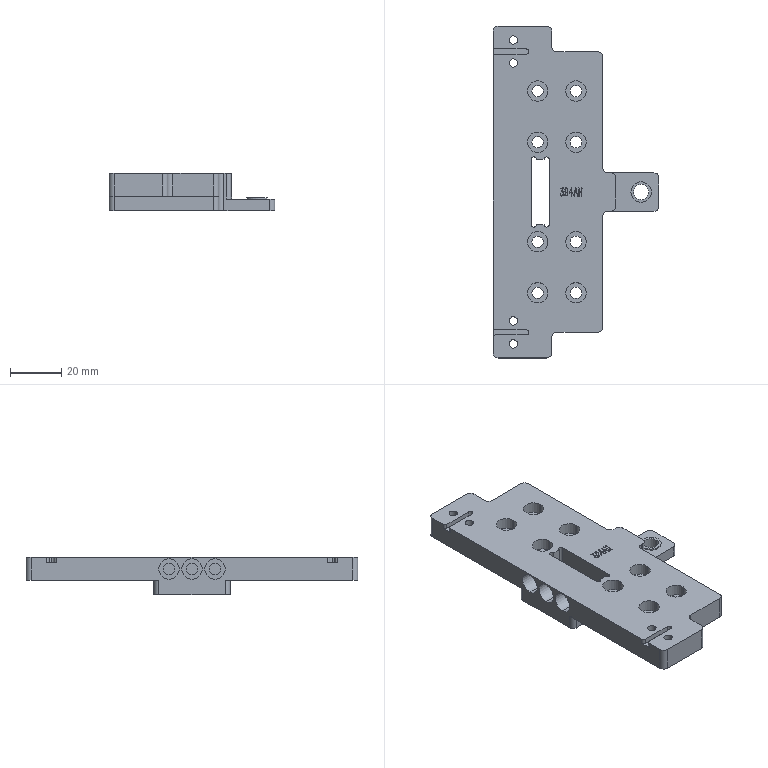NC program | NX | posted with a generic post | part box 65 x 130 x 14.5 mm
Lines 2037 to 2961 of 11541:
(ZLEVEL_PROFILE_COPY_COPY_COPY_1 , TOOL : D3)
N4036 T16 M6
N4038 G54
N4040 G17 G0 G90 X9.873 Y12.6 B0. C0. S9500 M3
N4042 G43 Z30. H16
N4044 Z-0.149
N4046 G94 G1 X10.133 Y12.15 F1000.
N4048 G3 X10.393 Y12. R0.3
N4050 G1 X11.336 F1200.
N4052 G2 X11.25 Y12.5 R1.5
N4054 G1 Y12.876
N4056 G3 X11.1 Y13.136 R0.3
N4058 G1 X10.65 Y13.396
N4060 G0 X9.873 Y12.6 Z-0.299
N4062 G1 X10.133 Y12.15 F1000.
N4064 G3 X10.393 Y12. R0.3
N4066 G1 X11.336 F1200.
N4068 G2 X11.25 Y12.5 R1.5
N4070 G1 Y12.876
N4072 G3 X11.1 Y13.136 R0.3
N4074 G1 X10.65 Y13.396
N4076 G0 X9.873 Y12.6 Z-0.448
N4078 G1 X10.133 Y12.15 F1000.
N4080 G3 X10.393 Y12. R0.3
N4082 G1 X11.336 F1200.
N4084 G2 X11.25 Y12.5 R1.5
N4086 G1 Y12.876
N4088 G3 X11.1 Y13.136 R0.3
N4090 G1 X10.65 Y13.396
N4092 G0 X9.873 Y12.6 Z-0.598
N4094 G1 X10.133 Y12.15 F1000.
N4096 G3 X10.393 Y12. R0.3
N4098 G1 X11.336 F1200.
N4100 G2 X11.25 Y12.5 R1.5
N4102 G1 Y12.876
N4104 G3 X11.1 Y13.136 R0.3
N4106 G1 X10.65 Y13.396
N4108 G0 X9.873 Y12.6 Z-0.747
N4110 G1 X10.133 Y12.15 F1000.
N4112 G3 X10.393 Y12. R0.3
N4114 G1 X11.336 F1200.
N4116 G2 X11.25 Y12.5 R1.5
N4118 G1 Y12.876
N4120 G3 X11.1 Y13.136 R0.3
N4122 G1 X10.65 Y13.396
N4124 G0 X9.873 Y12.6 Z-0.897
N4126 G1 X10.133 Y12.15 F1000.
N4128 G3 X10.393 Y12. R0.3
N4130 G1 X11.336 F1200.
N4132 G2 X11.25 Y12.5 R1.5
N4134 G1 Y12.876
N4136 G3 X11.1 Y13.136 R0.3
N4138 G1 X10.65 Y13.396
N4140 G0 X9.873 Y12.6 Z-1.046
N4142 G1 X10.133 Y12.15 F1000.
N4144 G3 X10.393 Y12. R0.3
N4146 G1 X11.336 F1200.
N4148 G2 X11.25 Y12.5 R1.5
N4150 G1 Y12.876
N4152 G3 X11.1 Y13.136 R0.3
N4154 G1 X10.65 Y13.396
N4156 G0 X9.873 Y12.6 Z-1.196
N4158 G1 X10.133 Y12.15 F1000.
N4160 G3 X10.393 Y12. R0.3
N4162 G1 X11.336 F1200.
N4164 G2 X11.25 Y12.5 R1.5
N4166 G1 Y12.876
N4168 G3 X11.1 Y13.136 R0.3
N4170 G1 X10.65 Y13.396
N4172 G0 X9.873 Y12.6 Z-1.345
N4174 G1 X10.133 Y12.15 F1000.
N4176 G3 X10.393 Y12. R0.3
N4178 G1 X11.336 F1200.
N4180 G2 X11.25 Y12.5 R1.5
N4182 G1 Y12.876
N4184 G3 X11.1 Y13.136 R0.3
N4186 G1 X10.65 Y13.396
N4188 G0 X9.873 Y12.6 Z-1.495
N4190 G1 X10.133 Y12.15 F1000.
N4192 G3 X10.393 Y12. R0.3
N4194 G1 X11.336 F1200.
N4196 G2 X11.25 Y12.5 R1.5
N4198 G1 Y12.876
N4200 G3 X11.1 Y13.136 R0.3
N4202 G1 X10.65 Y13.396
N4204 G0 X9.873 Y12.6 Z-1.644
N4206 G1 X10.133 Y12.15 F1000.
N4208 G3 X10.393 Y12. R0.3
N4210 G1 X11.336 F1200.
N4212 G2 X11.25 Y12.5 R1.5
N4214 G1 Y12.876
N4216 G3 X11.1 Y13.136 R0.3
N4218 G1 X10.65 Y13.396
N4220 G0 X9.873 Y12.6 Z-1.794
N4222 G1 X10.133 Y12.15 F1000.
N4224 G3 X10.393 Y12. R0.3
N4226 G1 X11.336 F1200.
N4228 G2 X11.25 Y12.5 R1.5
N4230 G1 Y12.876
N4232 G3 X11.1 Y13.136 R0.3
N4234 G1 X10.65 Y13.396
N4236 G0 X9.873 Y12.6 Z-1.943
N4238 G1 X10.133 Y12.15 F1000.
N4240 G3 X10.393 Y12. R0.3
N4242 G1 X11.336 F1200.
N4244 G2 X11.25 Y12.5 R1.5
N4246 G1 Y12.876
N4248 G3 X11.1 Y13.136 R0.3
N4250 G1 X10.65 Y13.396
N4252 G0 X9.873 Y12.6 Z-2.093
N4254 G1 X10.133 Y12.15 F1000.
N4256 G3 X10.393 Y12. R0.3
N4258 G1 X11.336 F1200.
N4260 G2 X11.25 Y12.5 R1.5
N4262 G1 Y12.876
N4264 G3 X11.1 Y13.136 R0.3
N4266 G1 X10.65 Y13.396
N4268 G0 X9.873 Y12.6 Z-2.242
N4270 G1 X10.133 Y12.15 F1000.
N4272 G3 X10.393 Y12. R0.3
N4274 G1 X11.336 F1200.
N4276 G2 X11.25 Y12.5 R1.5
N4278 G1 Y12.876
N4280 G3 X11.1 Y13.136 R0.3
N4282 G1 X10.65 Y13.396
N4284 G0 X9.873 Y12.6 Z-2.392
N4286 G1 X10.133 Y12.15 F1000.
N4288 G3 X10.393 Y12. R0.3
N4290 G1 X11.336 F1200.
N4292 G2 X11.25 Y12.5 R1.5
N4294 G1 Y12.876
N4296 G3 X11.1 Y13.136 R0.3
N4298 G1 X10.65 Y13.396
N4300 G0 X9.873 Y12.6 Z-2.541
N4302 G1 X10.133 Y12.15 F1000.
N4304 G3 X10.393 Y12. R0.3
N4306 G1 X11.336 F1200.
N4308 G2 X11.25 Y12.5 R1.5
N4310 G1 Y12.876
N4312 G3 X11.1 Y13.136 R0.3
N4314 G1 X10.65 Y13.396
N4316 G0 X9.873 Y12.6 Z-2.691
N4318 G1 X10.133 Y12.15 F1000.
N4320 G3 X10.393 Y12. R0.3
N4322 G1 X11.336 F1200.
N4324 G2 X11.25 Y12.5 R1.5
N4326 G1 Y12.876
N4328 G3 X11.1 Y13.136 R0.3
N4330 G1 X10.65 Y13.396
N4332 G0 X9.873 Y12.6 Z-2.84
N4334 G1 X10.133 Y12.15 F1000.
N4336 G3 X10.393 Y12. R0.3
N4338 G1 X11.336 F1200.
N4340 G2 X11.25 Y12.5 R1.5
N4342 G1 Y12.876
N4344 G3 X11.1 Y13.136 R0.3
N4346 G1 X10.65 Y13.396
N4348 G0 X9.873 Y12.6 Z-2.99
N4350 G1 X10.133 Y12.15 F1000.
N4352 G3 X10.393 Y12. R0.3
N4354 G1 X11.336 F1200.
N4356 G2 X11.25 Y12.5 R1.5
N4358 G1 Y12.876
N4360 G3 X11.1 Y13.136 R0.3
N4362 G1 X10.65 Y13.396
N4364 G0 X9.873 Y12.6 Z-3.139
N4366 G1 X10.133 Y12.15 F1000.
N4368 G3 X10.393 Y12. R0.3
N4370 G1 X11.336 F1200.
N4372 G2 X11.25 Y12.5 R1.5
N4374 G1 Y12.876
N4376 G3 X11.1 Y13.136 R0.3
N4378 G1 X10.65 Y13.396
N4380 G0 X9.873 Y12.6 Z-3.289
N4382 G1 X10.133 Y12.15 F1000.
N4384 G3 X10.393 Y12. R0.3
N4386 G1 X11.336 F1200.
N4388 G2 X11.25 Y12.5 R1.5
N4390 G1 Y12.876
N4392 G3 X11.1 Y13.136 R0.3
N4394 G1 X10.65 Y13.396
N4396 G0 X9.873 Y12.6 Z-3.438
N4398 G1 X10.133 Y12.15 F1000.
N4400 G3 X10.393 Y12. R0.3
N4402 G1 X11.336 F1200.
N4404 G2 X11.25 Y12.5 R1.5
N4406 G1 Y12.876
N4408 G3 X11.1 Y13.136 R0.3
N4410 G1 X10.65 Y13.396
N4412 G0 X9.873 Y12.6 Z-3.588
N4414 G1 X10.133 Y12.15 F1000.
N4416 G3 X10.393 Y12. R0.3
N4418 G1 X11.336 F1200.
N4420 G2 X11.25 Y12.5 R1.5
N4422 G1 Y12.876
N4424 G3 X11.1 Y13.136 R0.3
N4426 G1 X10.65 Y13.396
N4428 G0 X9.873 Y12.6 Z-3.737
N4430 G1 X10.133 Y12.15 F1000.
N4432 G3 X10.393 Y12. R0.3
N4434 G1 X11.336 F1200.
N4436 G2 X11.25 Y12.5 R1.5
N4438 G1 Y12.876
N4440 G3 X11.1 Y13.136 R0.3
N4442 G1 X10.65 Y13.396
N4444 G0 X9.873 Y12.6 Z-3.887
N4446 G1 X10.133 Y12.15 F1000.
N4448 G3 X10.393 Y12. R0.3
N4450 G1 X11.336 F1200.
N4452 G2 X11.25 Y12.5 R1.5
N4454 G1 Y12.876
N4456 G3 X11.1 Y13.136 R0.3
N4458 G1 X10.65 Y13.396
N4460 G0 X9.873 Y12.6 Z-4.036
N4462 G1 X10.133 Y12.15 F1000.
N4464 G3 X10.393 Y12. R0.3
N4466 G1 X11.336 F1200.
N4468 G2 X11.25 Y12.5 R1.5
N4470 G1 Y12.876
N4472 G3 X11.1 Y13.136 R0.3
N4474 G1 X10.65 Y13.396
N4476 G0 X9.873 Y12.6 Z-4.186
N4478 G1 X10.133 Y12.15 F1000.
N4480 G3 X10.393 Y12. R0.3
N4482 G1 X11.336 F1200.
N4484 G2 X11.25 Y12.5 R1.5
N4486 G1 Y12.876
N4488 G3 X11.1 Y13.136 R0.3
N4490 G1 X10.65 Y13.396
N4492 G0 X9.873 Y12.6 Z-4.335
N4494 G1 X10.133 Y12.15 F1000.
N4496 G3 X10.393 Y12. R0.3
N4498 G1 X11.336 F1200.
N4500 G2 X11.25 Y12.5 R1.5
N4502 G1 Y12.876
N4504 G3 X11.1 Y13.136 R0.3
N4506 G1 X10.65 Y13.396
N4508 G0 X9.873 Y12.6 Z-4.485
N4510 G1 X10.133 Y12.15 F1000.
N4512 G3 X10.393 Y12. R0.3
N4514 G1 X11.336 F1200.
N4516 G2 X11.25 Y12.5 R1.5
N4518 G1 Y12.876
N4520 G3 X11.1 Y13.136 R0.3
N4522 G1 X10.65 Y13.396
N4524 G0 X9.873 Y12.6 Z-4.634
N4526 G1 X10.133 Y12.15 F1000.
N4528 G3 X10.393 Y12. R0.3
N4530 G1 X11.336 F1200.
N4532 G2 X11.25 Y12.5 R1.5
N4534 G1 Y12.876
N4536 G3 X11.1 Y13.136 R0.3
N4538 G1 X10.65 Y13.396
N4540 G0 X9.873 Y12.6 Z-4.784
N4542 G1 X10.133 Y12.15 F1000.
N4544 G3 X10.393 Y12. R0.3
N4546 G1 X11.336 F1200.
N4548 G2 X11.25 Y12.5 R1.5
N4550 G1 Y12.876
N4552 G3 X11.1 Y13.136 R0.3
N4554 G1 X10.65 Y13.396
N4556 G0 X9.873 Y12.6 Z-4.933
N4558 G1 X10.133 Y12.15 F1000.
N4560 G3 X10.393 Y12. R0.3
N4562 G1 X11.336 F1200.
N4564 G2 X11.25 Y12.5 R1.5
N4566 G1 Y12.876
N4568 G3 X11.1 Y13.136 R0.3
N4570 G1 X10.65 Y13.396
N4572 G0 X9.873 Y12.6 Z-5.082
N4574 G1 X10.133 Y12.15 F1000.
N4576 G3 X10.393 Y12. R0.3
N4578 G1 X11.336 F1200.
N4580 G2 X11.25 Y12.5 R1.5
N4582 G1 Y12.876
N4584 G3 X11.1 Y13.136 R0.3
N4586 G1 X10.65 Y13.396
N4588 G0 X9.873 Y12.6 Z-5.232
N4590 G1 X10.133 Y12.15 F1000.
N4592 G3 X10.393 Y12. R0.3
N4594 G1 X11.336 F1200.
N4596 G2 X11.25 Y12.5 R1.5
N4598 G1 Y12.876
N4600 G3 X11.1 Y13.136 R0.3
N4602 G1 X10.65 Y13.396
N4604 G0 X9.873 Y12.6 Z-5.381
N4606 G1 X10.133 Y12.15 F1000.
N4608 G3 X10.393 Y12. R0.3
N4610 G1 X11.336 F1200.
N4612 G2 X11.25 Y12.5 R1.5
N4614 G1 Y12.876
N4616 G3 X11.1 Y13.136 R0.3
N4618 G1 X10.65 Y13.396
N4620 G0 X9.873 Y12.6 Z-5.531
N4622 G1 X10.133 Y12.15 F1000.
N4624 G3 X10.393 Y12. R0.3
N4626 G1 X11.336 F1200.
N4628 G2 X11.25 Y12.5 R1.5
N4630 G1 Y12.876
N4632 G3 X11.1 Y13.136 R0.3
N4634 G1 X10.65 Y13.396
N4636 G0 X9.873 Y12.6 Z-5.68
N4638 G1 X10.133 Y12.15 F1000.
N4640 G3 X10.393 Y12. R0.3
N4642 G1 X11.336 F1200.
N4644 G2 X11.25 Y12.5 R1.5
N4646 G1 Y12.876
N4648 G3 X11.1 Y13.136 R0.3
N4650 G1 X10.65 Y13.396
N4652 G0 X9.873 Y12.6 Z-5.83
N4654 G1 X10.133 Y12.15 F1000.
N4656 G3 X10.393 Y12. R0.3
N4658 G1 X11.336 F1200.
N4660 G2 X11.25 Y12.5 R1.5
N4662 G1 Y12.876
N4664 G3 X11.1 Y13.136 R0.3
N4666 G1 X10.65 Y13.396
N4668 G0 X9.873 Y12.6 Z-5.979
N4670 G1 X10.133 Y12.15 F1000.
N4672 G3 X10.393 Y12. R0.3
N4674 G1 X11.336 F1200.
N4676 G2 X11.25 Y12.5 R1.5
N4678 G1 Y12.876
N4680 G3 X11.1 Y13.136 R0.3
N4682 G1 X10.65 Y13.396
N4684 G0 X9.873 Y12.6 Z-6.129
N4686 G1 X10.133 Y12.15 F1000.
N4688 G3 X10.393 Y12. R0.3
N4690 G1 X11.336 F1200.
N4692 G2 X11.25 Y12.5 R1.5
N4694 G1 Y12.876
N4696 G3 X11.1 Y13.136 R0.3
N4698 G1 X10.65 Y13.396
N4700 G0 X9.873 Y12.6 Z-6.278
N4702 G1 X10.133 Y12.15 F1000.
N4704 G3 X10.393 Y12. R0.3
N4706 G1 X11.336 F1200.
N4708 G2 X11.25 Y12.5 R1.5
N4710 G1 Y12.876
N4712 G3 X11.1 Y13.136 R0.3
N4714 G1 X10.65 Y13.396
N4716 G0 X9.873 Y12.6 Z-6.428
N4718 G1 X10.133 Y12.15 F1000.
N4720 G3 X10.393 Y12. R0.3
N4722 G1 X11.336 F1200.
N4724 G2 X11.25 Y12.5 R1.5
N4726 G1 Y12.876
N4728 G3 X11.1 Y13.136 R0.3
N4730 G1 X10.65 Y13.396
N4732 G0 X9.873 Y12.6 Z-6.577
N4734 G1 X10.133 Y12.15 F1000.
N4736 G3 X10.393 Y12. R0.3
N4738 G1 X11.336 F1200.
N4740 G2 X11.25 Y12.5 R1.5
N4742 G1 Y12.876
N4744 G3 X11.1 Y13.136 R0.3
N4746 G1 X10.65 Y13.396
N4748 G0 X9.873 Y12.6 Z-6.727
N4750 G1 X10.133 Y12.15 F1000.
N4752 G3 X10.393 Y12. R0.3
N4754 G1 X11.336 F1200.
N4756 G2 X11.25 Y12.5 R1.5
N4758 G1 Y12.876
N4760 G3 X11.1 Y13.136 R0.3
N4762 G1 X10.65 Y13.396
N4764 G0 X9.873 Y12.6 Z-6.876
N4766 G1 X10.133 Y12.15 F1000.
N4768 G3 X10.393 Y12. R0.3
N4770 G1 X11.336 F1200.
N4772 G2 X11.25 Y12.5 R1.5
N4774 G1 Y12.876
N4776 G3 X11.1 Y13.136 R0.3
N4778 G1 X10.65 Y13.396
N4780 G0 X9.873 Y12.6 Z-7.026
N4782 G1 X10.133 Y12.15 F1000.
N4784 G3 X10.393 Y12. R0.3
N4786 G1 X11.336 F1200.
N4788 G2 X11.25 Y12.5 R1.5
N4790 G1 Y12.876
N4792 G3 X11.1 Y13.136 R0.3
N4794 G1 X10.65 Y13.396
N4796 G0 X9.873 Y12.6 Z-7.175
N4798 G1 X10.133 Y12.15 F1000.
N4800 G3 X10.393 Y12. R0.3
N4802 G1 X11.336 F1200.
N4804 G2 X11.25 Y12.5 R1.5
N4806 G1 Y12.876
N4808 G3 X11.1 Y13.136 R0.3
N4810 G1 X10.65 Y13.396
N4812 G0 X9.873 Y12.6 Z-7.325
N4814 G1 X10.133 Y12.15 F1000.
N4816 G3 X10.393 Y12. R0.3
N4818 G1 X11.336 F1200.
N4820 G2 X11.25 Y12.5 R1.5
N4822 G1 Y12.876
N4824 G3 X11.1 Y13.136 R0.3
N4826 G1 X10.65 Y13.396
N4828 G0 X9.873 Y12.6 Z-7.474
N4830 G1 X10.133 Y12.15 F1000.
N4832 G3 X10.393 Y12. R0.3
N4834 G1 X11.336 F1200.
N4836 G2 X11.25 Y12.5 R1.5
N4838 G1 Y12.876
N4840 G3 X11.1 Y13.136 R0.3
N4842 G1 X10.65 Y13.396
N4844 G0 X9.873 Y12.6 Z-7.624
N4846 G1 X10.133 Y12.15 F1000.
N4848 G3 X10.393 Y12. R0.3
N4850 G1 X11.336 F1200.
N4852 G2 X11.25 Y12.5 R1.5
N4854 G1 Y12.876
N4856 G3 X11.1 Y13.136 R0.3
N4858 G1 X10.65 Y13.396
N4860 G0 X9.873 Y12.6 Z-7.773
N4862 G1 X10.133 Y12.15 F1000.
N4864 G3 X10.393 Y12. R0.3
N4866 G1 X11.336 F1200.
N4868 G2 X11.25 Y12.5 R1.5
N4870 G1 Y12.876
N4872 G3 X11.1 Y13.136 R0.3
N4874 G1 X10.65 Y13.396
N4876 G0 X9.873 Y12.6 Z-7.923
N4878 G1 X10.133 Y12.15 F1000.
N4880 G3 X10.393 Y12. R0.3
N4882 G1 X11.336 F1200.
N4884 G2 X11.25 Y12.5 R1.5
N4886 G1 Y12.876
N4888 G3 X11.1 Y13.136 R0.3
N4890 G1 X10.65 Y13.396
N4892 G0 X9.873 Y12.6 Z-8.072
N4894 G1 X10.133 Y12.15 F1000.
N4896 G3 X10.393 Y12. R0.3
N4898 G1 X11.336 F1200.
N4900 G2 X11.25 Y12.5 R1.5
N4902 G1 Y12.876
N4904 G3 X11.1 Y13.136 R0.3
N4906 G1 X10.65 Y13.396
N4908 G0 X9.873 Y12.6 Z-8.222
N4910 G1 X10.133 Y12.15 F1000.
N4912 G3 X10.393 Y12. R0.3
N4914 G1 X11.336 F1200.
N4916 G2 X11.25 Y12.5 R1.5
N4918 G1 Y12.876
N4920 G3 X11.1 Y13.136 R0.3
N4922 G1 X10.65 Y13.396
N4924 G0 X9.873 Y12.6 Z-8.371
N4926 G1 X10.133 Y12.15 F1000.
N4928 G3 X10.393 Y12. R0.3
N4930 G1 X11.336 F1200.
N4932 G2 X11.25 Y12.5 R1.5
N4934 G1 Y12.876
N4936 G3 X11.1 Y13.136 R0.3
N4938 G1 X10.65 Y13.396
N4940 G0 X9.873 Y12.6 Z-8.521
N4942 G1 X10.133 Y12.15 F1000.
N4944 G3 X10.393 Y12. R0.3
N4946 G1 X11.336 F1200.
N4948 G2 X11.25 Y12.5 R1.5
N4950 G1 Y12.876
N4952 G3 X11.1 Y13.136 R0.3
N4954 G1 X10.65 Y13.396
N4956 G0 X9.873 Y12.6 Z-8.67
N4958 G1 X10.133 Y12.15 F1000.
N4960 G3 X10.393 Y12. R0.3
N4962 G1 X11.336 F1200.
N4964 G2 X11.25 Y12.5 R1.5
N4966 G1 Y12.876
N4968 G3 X11.1 Y13.136 R0.3
N4970 G1 X10.65 Y13.396
N4972 G0 X9.873 Y12.6 Z-8.82
N4974 G1 X10.133 Y12.15 F1000.
N4976 G3 X10.393 Y12. R0.3
N4978 G1 X11.336 F1200.
N4980 G2 X11.25 Y12.5 R1.5
N4982 G1 Y12.876
N4984 G3 X11.1 Y13.136 R0.3
N4986 G1 X10.65 Y13.396
N4988 G0 X9.873 Y12.6 Z-8.969
N4990 G1 X10.133 Y12.15 F1000.
N4992 G3 X10.393 Y12. R0.3
N4994 G1 X11.336 F1200.
N4996 G2 X11.25 Y12.5 R1.5
N4998 G1 Y12.876
N5000 G3 X11.1 Y13.136 R0.3
N5002 G1 X10.65 Y13.396
N5004 G0 X9.873 Y12.6 Z-9.119
N5006 G1 X10.133 Y12.15 F1000.
N5008 G3 X10.393 Y12. R0.3
N5010 G1 X11.336 F1200.
N5012 G2 X11.25 Y12.5 R1.5
N5014 G1 Y12.876
N5016 G3 X11.1 Y13.136 R0.3
N5018 G1 X10.65 Y13.396
N5020 G0 X9.873 Y12.6 Z-9.268
N5022 G1 X10.133 Y12.15 F1000.
N5024 G3 X10.393 Y12. R0.3
N5026 G1 X11.336 F1200.
N5028 G2 X11.25 Y12.5 R1.5
N5030 G1 Y12.876
N5032 G3 X11.1 Y13.136 R0.3
N5034 G1 X10.65 Y13.396
N5036 G0 X9.873 Y12.6 Z-9.418
N5038 G1 X10.133 Y12.15 F1000.
N5040 G3 X10.393 Y12. R0.3
N5042 G1 X11.336 F1200.
N5044 G2 X11.25 Y12.5 R1.5
N5046 G1 Y12.876
N5048 G3 X11.1 Y13.136 R0.3
N5050 G1 X10.65 Y13.396
N5052 G0 X9.873 Y12.6 Z-9.567
N5054 G1 X10.133 Y12.15 F1000.
N5056 G3 X10.393 Y12. R0.3
N5058 G1 X11.336 F1200.
N5060 G2 X11.25 Y12.5 R1.5
N5062 G1 Y12.876
N5064 G3 X11.1 Y13.136 R0.3
N5066 G1 X10.65 Y13.396
N5068 G0 X9.873 Y12.6 Z-9.716
N5070 G1 X10.133 Y12.15 F1000.
N5072 G3 X10.393 Y12. R0.3
N5074 G1 X11.336 F1200.
N5076 G2 X11.25 Y12.5 R1.5
N5078 G1 Y12.876
N5080 G3 X11.1 Y13.136 R0.3
N5082 G1 X10.65 Y13.396
N5084 G0 X9.873 Y12.6 Z-9.866
N5086 G1 X10.133 Y12.15 F1000.
N5088 G3 X10.393 Y12. R0.3
N5090 G1 X11.336 F1200.
N5092 G2 X11.25 Y12.5 R1.5
N5094 G1 Y12.876
N5096 G3 X11.1 Y13.136 R0.3
N5098 G1 X10.65 Y13.396
N5100 G0 X9.873 Y12.6 Z-10.015
N5102 G1 X10.133 Y12.15 F1000.
N5104 G3 X10.393 Y12. R0.3
N5106 G1 X11.336 F1200.
N5108 G2 X11.25 Y12.5 R1.5
N5110 G1 Y12.876
N5112 G3 X11.1 Y13.136 R0.3
N5114 G1 X10.65 Y13.396
N5116 G0 X9.873 Y12.6 Z-10.165
N5118 G1 X10.133 Y12.15 F1000.
N5120 G3 X10.393 Y12. R0.3
N5122 G1 X11.336 F1200.
N5124 G2 X11.25 Y12.5 R1.5
N5126 G1 Y12.876
N5128 G3 X11.1 Y13.136 R0.3
N5130 G1 X10.65 Y13.396
N5132 G0 X9.873 Y12.6 Z-10.314
N5134 G1 X10.133 Y12.15 F1000.
N5136 G3 X10.393 Y12. R0.3
N5138 G1 X11.336 F1200.
N5140 G2 X11.25 Y12.5 R1.5
N5142 G1 Y12.876
N5144 G3 X11.1 Y13.136 R0.3
N5146 G1 X10.65 Y13.396
N5148 G0 X9.873 Y12.6 Z-10.464
N5150 G1 X10.133 Y12.15 F1000.
N5152 G3 X10.393 Y12. R0.3
N5154 G1 X11.336 F1200.
N5156 G2 X11.25 Y12.5 R1.5
N5158 G1 Y12.876
N5160 G3 X11.1 Y13.136 R0.3
N5162 G1 X10.65 Y13.396
N5164 G0 X9.873 Y12.6 Z-10.613
N5166 G1 X10.133 Y12.15 F1000.
N5168 G3 X10.393 Y12. R0.3
N5170 G1 X11.336 F1200.
N5172 G2 X11.25 Y12.5 R1.5
N5174 G1 Y12.876
N5176 G3 X11.1 Y13.136 R0.3
N5178 G1 X10.65 Y13.396
N5180 G0 X9.873 Y12.6 Z-10.763
N5182 G1 X10.133 Y12.15 F1000.
N5184 G3 X10.393 Y12. R0.3
N5186 G1 X11.336 F1200.
N5188 G2 X11.25 Y12.5 R1.5
N5190 G1 Y12.876
N5192 G3 X11.1 Y13.136 R0.3
N5194 G1 X10.65 Y13.396
N5196 G0 X9.873 Y12.6 Z-10.912
N5198 G1 X10.133 Y12.15 F1000.
N5200 G3 X10.393 Y12. R0.3
N5202 G1 X11.336 F1200.
N5204 G2 X11.25 Y12.5 R1.5
N5206 G1 Y12.876
N5208 G3 X11.1 Y13.136 R0.3
N5210 G1 X10.65 Y13.396
N5212 G0 X9.873 Y12.6 Z-11.062
N5214 G1 X10.133 Y12.15 F1000.
N5216 G3 X10.393 Y12. R0.3
N5218 G1 X11.336 F1200.
N5220 G2 X11.25 Y12.5 R1.5
N5222 G1 Y12.876
N5224 G3 X11.1 Y13.136 R0.3
N5226 G1 X10.65 Y13.396
N5228 G0 X9.873 Y12.6 Z-11.211
N5230 G1 X10.133 Y12.15 F1000.
N5232 G3 X10.393 Y12. R0.3
N5234 G1 X11.336 F1200.
N5236 G2 X11.25 Y12.5 R1.5
N5238 G1 Y12.876
N5240 G3 X11.1 Y13.136 R0.3
N5242 G1 X10.65 Y13.396
N5244 G0 X9.873 Y12.6 Z-11.361
N5246 G1 X10.133 Y12.15 F1000.
N5248 G3 X10.393 Y12. R0.3
N5250 G1 X11.336 F1200.
N5252 G2 X11.25 Y12.5 R1.5
N5254 G1 Y12.876
N5256 G3 X11.1 Y13.136 R0.3
N5258 G1 X10.65 Y13.396
N5260 G0 X9.873 Y12.6 Z-11.51
N5262 G1 X10.133 Y12.15 F1000.
N5264 G3 X10.393 Y12. R0.3
N5266 G1 X11.336 F1200.
N5268 G2 X11.25 Y12.5 R1.5
N5270 G1 Y12.876
N5272 G3 X11.1 Y13.136 R0.3
N5274 G1 X10.65 Y13.396
N5276 G0 X9.873 Y12.6 Z-11.66
N5278 G1 X10.133 Y12.15 F1000.
N5280 G3 X10.393 Y12. R0.3
N5282 G1 X11.336 F1200.
N5284 G2 X11.25 Y12.5 R1.5
N5286 G1 Y12.876
N5288 G3 X11.1 Y13.136 R0.3
N5290 G1 X10.65 Y13.396
N5292 G0 X9.873 Y12.6 Z-11.809
N5294 G1 X10.133 Y12.15 F1000.
N5296 G3 X10.393 Y12. R0.3
N5298 G1 X11.336 F1200.
N5300 G2 X11.25 Y12.5 R1.5
N5302 G1 Y12.876
N5304 G3 X11.1 Y13.136 R0.3
N5306 G1 X10.65 Y13.396
N5308 G0 X9.873 Y12.6 Z-11.959
N5310 G1 X10.133 Y12.15 F1000.
N5312 G3 X10.393 Y12. R0.3
N5314 G1 X11.336 F1200.
N5316 G2 X11.25 Y12.5 R1.5
N5318 G1 Y12.876
N5320 G3 X11.1 Y13.136 R0.3
N5322 G1 X10.65 Y13.396
N5324 G0 X9.873 Y12.6 Z-12.108
N5326 G1 X10.133 Y12.15 F1000.
N5328 G3 X10.393 Y12. R0.3
N5330 G1 X11.336 F1200.
N5332 G2 X11.25 Y12.5 R1.5
N5334 G1 Y12.876
N5336 G3 X11.1 Y13.136 R0.3
N5338 G1 X10.65 Y13.396
N5340 G0 X9.873 Y12.6 Z-12.258
N5342 G1 X10.133 Y12.15 F1000.
N5344 G3 X10.393 Y12. R0.3
N5346 G1 X11.336 F1200.
N5348 G2 X11.25 Y12.5 R1.5
N5350 G1 Y12.876
N5352 G3 X11.1 Y13.136 R0.3
N5354 G1 X10.65 Y13.396
N5356 G0 X9.873 Y12.6 Z-12.407
N5358 G1 X10.133 Y12.15 F1000.
N5360 G3 X10.393 Y12. R0.3
N5362 G1 X11.336 F1200.
N5364 G2 X11.25 Y12.5 R1.5
N5366 G1 Y12.876
N5368 G3 X11.1 Y13.136 R0.3
N5370 G1 X10.65 Y13.396
N5372 G0 X9.873 Y12.6 Z-12.557
N5374 G1 X10.133 Y12.15 F1000.
N5376 G3 X10.393 Y12. R0.3
N5378 G1 X11.336 F1200.
N5380 G2 X11.25 Y12.5 R1.5
N5382 G1 Y12.876
N5384 G3 X11.1 Y13.136 R0.3
N5386 G1 X10.65 Y13.396
N5388 G0 X9.873 Y12.6 Z-12.706
N5390 G1 X10.133 Y12.15 F1000.
N5392 G3 X10.393 Y12. R0.3
N5394 G1 X11.336 F1200.
N5396 G2 X11.25 Y12.5 R1.5
N5398 G1 Y12.876
N5400 G3 X11.1 Y13.136 R0.3
N5402 G1 X10.65 Y13.396
N5404 G0 X9.873 Y12.6 Z-12.856
N5406 G1 X10.133 Y12.15 F1000.
N5408 G3 X10.393 Y12. R0.3
N5410 G1 X11.336 F1200.
N5412 G2 X11.25 Y12.5 R1.5
N5414 G1 Y12.876
N5416 G3 X11.1 Y13.136 R0.3
N5418 G1 X10.65 Y13.396
N5420 G0 X9.873 Y12.6 Z-13.005
N5422 G1 X10.133 Y12.15 F1000.
N5424 G3 X10.393 Y12. R0.3
N5426 G1 X11.336 F1200.
N5428 G2 X11.25 Y12.5 R1.5
N5430 G1 Y12.876
N5432 G3 X11.1 Y13.136 R0.3
N5434 G1 X10.65 Y13.396
N5436 G0 X9.873 Y12.6 Z-13.155
N5438 G1 X10.133 Y12.15 F1000.
N5440 G3 X10.393 Y12. R0.3
N5442 G1 X11.336 F1200.
N5444 G2 X11.25 Y12.5 R1.5
N5446 G1 Y12.876
N5448 G3 X11.1 Y13.136 R0.3
N5450 G1 X10.65 Y13.396
N5452 G0 X9.873 Y12.6 Z-13.304
N5454 G1 X10.133 Y12.15 F1000.
N5456 G3 X10.393 Y12. R0.3
N5458 G1 X11.336 F1200.
N5460 G2 X11.25 Y12.5 R1.5
N5462 G1 Y12.876
N5464 G3 X11.1 Y13.136 R0.3
N5466 G1 X10.65 Y13.396
N5468 G0 X9.873 Y12.6 Z-13.454
N5470 G1 X10.133 Y12.15 F1000.
N5472 G3 X10.393 Y12. R0.3
N5474 G1 X11.336 F1200.
N5476 G2 X11.25 Y12.5 R1.5
N5478 G1 Y12.876
N5480 G3 X11.1 Y13.136 R0.3
N5482 G1 X10.65 Y13.396
N5484 G0 X9.873 Y12.6 Z-13.603
N5486 G1 X10.133 Y12.15 F1000.
N5488 G3 X10.393 Y12. R0.3
N5490 G1 X11.336 F1200.
N5492 G2 X11.25 Y12.5 R1.5
N5494 G1 Y12.876
N5496 G3 X11.1 Y13.136 R0.3
N5498 G1 X10.65 Y13.396
N5500 G0 X9.873 Y12.6 Z-13.753
N5502 G1 X10.133 Y12.15 F1000.
N5504 G3 X10.393 Y12. R0.3
N5506 G1 X11.336 F1200.
N5508 G2 X11.25 Y12.5 R1.5
N5510 G1 Y12.876
N5512 G3 X11.1 Y13.136 R0.3
N5514 G1 X10.65 Y13.396
N5516 G0 X9.873 Y12.6 Z-13.902
N5518 G1 X10.133 Y12.15 F1000.
N5520 G3 X10.393 Y12. R0.3
N5522 G1 X11.336 F1200.
N5524 G2 X11.25 Y12.5 R1.5
N5526 G1 Y12.876
N5528 G3 X11.1 Y13.136 R0.3
N5530 G1 X10.65 Y13.396
N5532 G0 X9.873 Y12.6 Z-14.052
N5534 G1 X10.133 Y12.15 F1000.
N5536 G3 X10.393 Y12. R0.3
N5538 G1 X11.336 F1200.
N5540 G2 X11.25 Y12.5 R1.5
N5542 G1 Y12.876
N5544 G3 X11.1 Y13.136 R0.3
N5546 G1 X10.65 Y13.396
N5548 G0 X9.873 Y12.6 Z-14.201
N5550 G1 X10.133 Y12.15 F1000.
N5552 G3 X10.393 Y12. R0.3
N5554 G1 X11.336 F1200.
N5556 G2 X11.25 Y12.5 R1.5
N5558 G1 Y12.876
N5560 G3 X11.1 Y13.136 R0.3
N5562 G1 X10.65 Y13.396
N5564 G0 X9.873 Y12.6 Z-14.351
N5566 G1 X10.133 Y12.15 F1000.
N5568 G3 X10.393 Y12. R0.3
N5570 G1 X11.336 F1200.
N5572 G2 X11.25 Y12.5 R1.5
N5574 G1 Y12.876
N5576 G3 X11.1 Y13.136 R0.3
N5578 G1 X10.65 Y13.396
N5580 G0 X9.873 Y12.6 Z-14.5
N5582 G1 X10.133 Y12.15 F1000.
N5584 G3 X10.393 Y12. R0.3
N5586 G1 X11.336 F1200.
N5588 G2 X11.25 Y12.5 R1.5
N5590 G1 Y12.876
N5592 G3 X11.1 Y13.136 R0.3
N5594 G1 X10.65 Y13.396
N5596 G0 Z30.
N5598 Y14.604
N5600 Z-0.149
N5602 G1 X11.1 Y14.864 F1000.
N5604 G3 X11.25 Y15.124 R0.3
N5606 G1 Y15.5 F1200.
N5608 G2 X11.336 Y16. R1.5
N5610 G1 X10.393
N5612 G3 X10.133 Y15.85 R0.3
N5614 G1 X9.873 Y15.4
N5616 G0 X10.65 Y14.604 Z-0.299
N5618 G1 X11.1 Y14.864 F1000.
N5620 G3 X11.25 Y15.124 R0.3
N5622 G1 Y15.5 F1200.
N5624 G2 X11.336 Y16. R1.5
N5626 G1 X10.393
N5628 G3 X10.133 Y15.85 R0.3
N5630 G1 X9.873 Y15.4
N5632 G0 X10.65 Y14.604 Z-0.448
N5634 G1 X11.1 Y14.864 F1000.
N5636 G3 X11.25 Y15.124 R0.3
N5638 G1 Y15.5 F1200.
N5640 G2 X11.336 Y16. R1.5
N5642 G1 X10.393
N5644 G3 X10.133 Y15.85 R0.3
N5646 G1 X9.873 Y15.4
N5648 G0 X10.65 Y14.604 Z-0.598
N5650 G1 X11.1 Y14.864 F1000.
N5652 G3 X11.25 Y15.124 R0.3
N5654 G1 Y15.5 F1200.
N5656 G2 X11.336 Y16. R1.5
N5658 G1 X10.393
N5660 G3 X10.133 Y15.85 R0.3
N5662 G1 X9.873 Y15.4
N5664 G0 X10.65 Y14.604 Z-0.747
N5666 G1 X11.1 Y14.864 F1000.
N5668 G3 X11.25 Y15.124 R0.3
N5670 G1 Y15.5 F1200.
N5672 G2 X11.336 Y16. R1.5
N5674 G1 X10.393
N5676 G3 X10.133 Y15.85 R0.3
N5678 G1 X9.873 Y15.4
N5680 G0 X10.65 Y14.604 Z-0.897
N5682 G1 X11.1 Y14.864 F1000.
N5684 G3 X11.25 Y15.124 R0.3
N5686 G1 Y15.5 F1200.
N5688 G2 X11.336 Y16. R1.5
N5690 G1 X10.393
N5692 G3 X10.133 Y15.85 R0.3
N5694 G1 X9.873 Y15.4
N5696 G0 X10.65 Y14.604 Z-1.046
N5698 G1 X11.1 Y14.864 F1000.
N5700 G3 X11.25 Y15.124 R0.3
N5702 G1 Y15.5 F1200.
N5704 G2 X11.336 Y16. R1.5
N5706 G1 X10.393
N5708 G3 X10.133 Y15.85 R0.3
N5710 G1 X9.873 Y15.4
N5712 G0 X10.65 Y14.604 Z-1.196
N5714 G1 X11.1 Y14.864 F1000.
N5716 G3 X11.25 Y15.124 R0.3
N5718 G1 Y15.5 F1200.
N5720 G2 X11.336 Y16. R1.5
N5722 G1 X10.393
N5724 G3 X10.133 Y15.85 R0.3
N5726 G1 X9.873 Y15.4
N5728 G0 X10.65 Y14.604 Z-1.345
N5730 G1 X11.1 Y14.864 F1000.
N5732 G3 X11.25 Y15.124 R0.3
N5734 G1 Y15.5 F1200.
N5736 G2 X11.336 Y16. R1.5
N5738 G1 X10.393
N5740 G3 X10.133 Y15.85 R0.3
N5742 G1 X9.873 Y15.4
N5744 G0 X10.65 Y14.604 Z-1.495
N5746 G1 X11.1 Y14.864 F1000.
N5748 G3 X11.25 Y15.124 R0.3
N5750 G1 Y15.5 F1200.
N5752 G2 X11.336 Y16. R1.5
N5754 G1 X10.393
N5756 G3 X10.133 Y15.85 R0.3
N5758 G1 X9.873 Y15.4
N5760 G0 X10.65 Y14.604 Z-1.644
N5762 G1 X11.1 Y14.864 F1000.
N5764 G3 X11.25 Y15.124 R0.3
N5766 G1 Y15.5 F1200.
N5768 G2 X11.336 Y16. R1.5
N5770 G1 X10.393
N5772 G3 X10.133 Y15.85 R0.3
N5774 G1 X9.873 Y15.4
N5776 G0 X10.65 Y14.604 Z-1.794
N5778 G1 X11.1 Y14.864 F1000.
N5780 G3 X11.25 Y15.124 R0.3
N5782 G1 Y15.5 F1200.
N5784 G2 X11.336 Y16. R1.5
N5786 G1 X10.393
N5788 G3 X10.133 Y15.85 R0.3
N5790 G1 X9.873 Y15.4
N5792 G0 X10.65 Y14.604 Z-1.943
N5794 G1 X11.1 Y14.864 F1000.
N5796 G3 X11.25 Y15.124 R0.3
N5798 G1 Y15.5 F1200.
N5800 G2 X11.336 Y16. R1.5
N5802 G1 X10.393
N5804 G3 X10.133 Y15.85 R0.3
N5806 G1 X9.873 Y15.4
N5808 G0 X10.65 Y14.604 Z-2.093
N5810 G1 X11.1 Y14.864 F1000.
N5812 G3 X11.25 Y15.124 R0.3
N5814 G1 Y15.5 F1200.
N5816 G2 X11.336 Y16. R1.5
N5818 G1 X10.393
N5820 G3 X10.133 Y15.85 R0.3
N5822 G1 X9.873 Y15.4
N5824 G0 X10.65 Y14.604 Z-2.242
N5826 G1 X11.1 Y14.864 F1000.
N5828 G3 X11.25 Y15.124 R0.3
N5830 G1 Y15.5 F1200.
N5832 G2 X11.336 Y16. R1.5
N5834 G1 X10.393
N5836 G3 X10.133 Y15.85 R0.3
N5838 G1 X9.873 Y15.4
N5840 G0 X10.65 Y14.604 Z-2.392
N5842 G1 X11.1 Y14.864 F1000.
N5844 G3 X11.25 Y15.124 R0.3
N5846 G1 Y15.5 F1200.
N5848 G2 X11.336 Y16. R1.5
N5850 G1 X10.393
N5852 G3 X10.133 Y15.85 R0.3
N5854 G1 X9.873 Y15.4
N5856 G0 X10.65 Y14.604 Z-2.541
N5858 G1 X11.1 Y14.864 F1000.
N5860 G3 X11.25 Y15.124 R0.3
N5862 G1 Y15.5 F1200.
N5864 G2 X11.336 Y16. R1.5
N5866 G1 X10.393
N5868 G3 X10.133 Y15.85 R0.3
N5870 G1 X9.873 Y15.4
N5872 G0 X10.65 Y14.604 Z-2.691
N5874 G1 X11.1 Y14.864 F1000.
N5876 G3 X11.25 Y15.124 R0.3
N5878 G1 Y15.5 F1200.